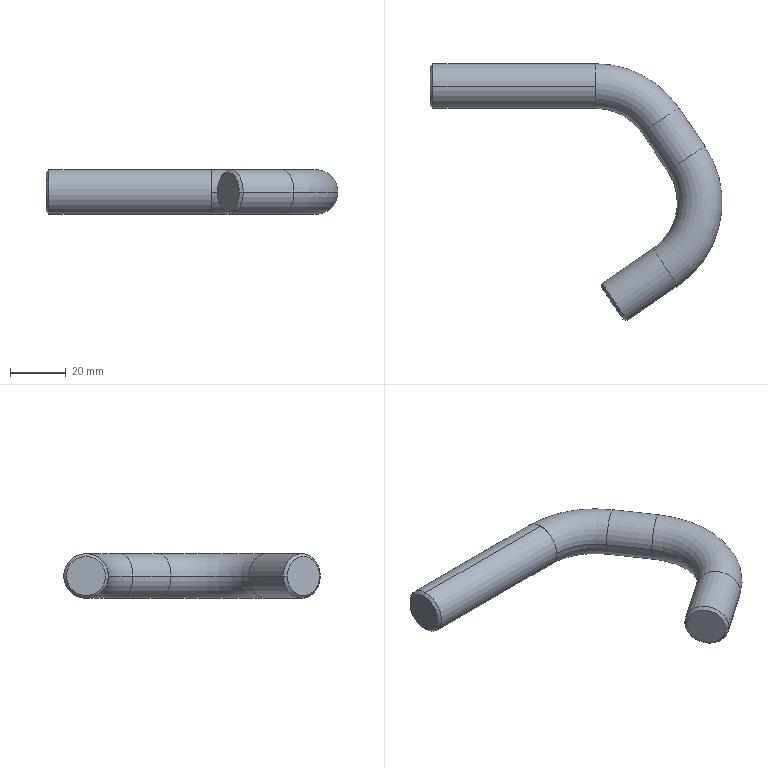Part | SolidWorks | features Chamfer 2, WeldMemberFeat 1, WeldmentFeature 1 | 5 solids | 24 faces | box 104.462 x 91.811 x 16 mm | volume 34123 mm3 | plane 10 | cylinder 6 | cone 4 | torus 4 | commonest cylinder face diameters 16 x6
STEP:
#1=CARTESIAN_POINT('',(0.,0.,7.));
#2=VERTEX_POINT('',#1);
#3=CARTESIAN_POINT('',(0.,0.,-7.));
#4=VERTEX_POINT('',#3);
#5=CARTESIAN_POINT('',(0.,0.,0.));
#6=DIRECTION('',(-1.,0.,0.));
#7=DIRECTION('',(0.,0.,1.));
#8=AXIS2_PLACEMENT_3D('',#5,#6,#7);
#9=CIRCLE('',#8,7.);
#10=EDGE_CURVE('',#2,#4,#9,.T.);
#11=ORIENTED_EDGE('',*,*,#10,.F.);
#12=CARTESIAN_POINT('',(1.,0.,8.));
#13=VERTEX_POINT('',#12);
#14=CARTESIAN_POINT('',(0.,0.,7.));
#15=DIRECTION('',(0.7071,0.,0.7071));
#16=VECTOR('',#15,1000.);
#17=LINE('',#14,#16);
#18=EDGE_CURVE('',#2,#13,#17,.T.);
#19=ORIENTED_EDGE('',*,*,#18,.T.);
#20=CARTESIAN_POINT('',(1.,0.,-8.));
#21=VERTEX_POINT('',#20);
#22=CARTESIAN_POINT('',(1.,0.,0.));
#23=DIRECTION('',(1.,0.,0.));
#24=DIRECTION('',(0.,0.,1.));
#25=AXIS2_PLACEMENT_3D('',#22,#23,#24);
#26=CIRCLE('',#25,8.);
#27=EDGE_CURVE('',#21,#13,#26,.T.);
#28=ORIENTED_EDGE('',*,*,#27,.F.);
#29=CARTESIAN_POINT('',(0.,0.,-7.));
#30=DIRECTION('',(0.7071,0.,-0.7071));
#31=VECTOR('',#30,1000.);
#32=LINE('',#29,#31);
#33=EDGE_CURVE('',#4,#21,#32,.T.);
#34=ORIENTED_EDGE('',*,*,#33,.F.);
#35=EDGE_LOOP('',(#11,#19,#28,#34));
#36=FACE_OUTER_BOUND('',#35,.T.);
#37=CARTESIAN_POINT('',(0.,0.,0.));
#38=DIRECTION('',(1.,0.,0.));
#39=DIRECTION('',(0.,0.,-1.));
#40=AXIS2_PLACEMENT_3D('',#37,#38,#39);
#41=CONICAL_SURFACE('',#40,7.,0.7854);
#42=ADVANCED_FACE('',(#36),#41,.T.);
#43=ORIENTED_EDGE('',*,*,#27,.T.);
#44=CARTESIAN_POINT('',(59.174,0.,8.));
#45=VERTEX_POINT('',#44);
#46=CARTESIAN_POINT('',(0.,0.,8.));
#47=DIRECTION('',(1.,0.,0.));
#48=VECTOR('',#47,1000.);
#49=LINE('',#46,#48);
#50=EDGE_CURVE('',#13,#45,#49,.T.);
#51=ORIENTED_EDGE('',*,*,#50,.T.);
#52=CARTESIAN_POINT('',(59.174,0.,-8.));
#53=VERTEX_POINT('',#52);
#54=CARTESIAN_POINT('',(59.174,0.,0.));
#55=DIRECTION('',(-1.,0.,0.));
#56=DIRECTION('',(0.,0.,1.));
#57=AXIS2_PLACEMENT_3D('',#54,#55,#56);
#58=CIRCLE('',#57,8.);
#59=EDGE_CURVE('',#45,#53,#58,.T.);
#60=ORIENTED_EDGE('',*,*,#59,.T.);
#61=CARTESIAN_POINT('',(0.,0.,-8.));
#62=DIRECTION('',(1.,0.,0.));
#63=VECTOR('',#62,1000.);
#64=LINE('',#61,#63);
#65=EDGE_CURVE('',#21,#53,#64,.T.);
#66=ORIENTED_EDGE('',*,*,#65,.F.);
#67=EDGE_LOOP('',(#43,#51,#60,#66));
#68=FACE_OUTER_BOUND('',#67,.T.);
#69=CARTESIAN_POINT('',(0.,0.,0.));
#70=DIRECTION('',(1.,0.,0.));
#71=DIRECTION('',(0.,0.,-1.));
#72=AXIS2_PLACEMENT_3D('',#69,#70,#71);
#73=CYLINDRICAL_SURFACE('',#72,8.);
#74=ADVANCED_FACE('',(#68),#73,.T.);
#75=ORIENTED_EDGE('',*,*,#50,.F.);
#76=CARTESIAN_POINT('',(1.,0.,0.));
#77=DIRECTION('',(1.,0.,0.));
#78=DIRECTION('',(0.,0.,1.));
#79=AXIS2_PLACEMENT_3D('',#76,#77,#78);
#80=CIRCLE('',#79,8.);
#81=EDGE_CURVE('',#13,#21,#80,.T.);
#82=ORIENTED_EDGE('',*,*,#81,.T.);
#83=ORIENTED_EDGE('',*,*,#65,.T.);
#84=CARTESIAN_POINT('',(59.174,0.,0.));
#85=DIRECTION('',(-1.,0.,0.));
#86=DIRECTION('',(0.,0.,1.));
#87=AXIS2_PLACEMENT_3D('',#84,#85,#86);
#88=CIRCLE('',#87,8.);
#89=EDGE_CURVE('',#53,#45,#88,.T.);
#90=ORIENTED_EDGE('',*,*,#89,.T.);
#91=EDGE_LOOP('',(#75,#82,#83,#90));
#92=FACE_OUTER_BOUND('',#91,.T.);
#93=CARTESIAN_POINT('',(0.,0.,0.));
#94=DIRECTION('',(1.,0.,0.));
#95=DIRECTION('',(0.,0.,-1.));
#96=AXIS2_PLACEMENT_3D('',#93,#94,#95);
#97=CYLINDRICAL_SURFACE('',#96,8.);
#98=ADVANCED_FACE('',(#92),#97,.T.);
#99=CARTESIAN_POINT('',(0.,0.,0.));
#100=DIRECTION('',(-1.,0.,0.));
#101=DIRECTION('',(0.,0.,1.));
#102=AXIS2_PLACEMENT_3D('',#99,#100,#101);
#103=CIRCLE('',#102,7.);
#104=EDGE_CURVE('',#4,#2,#103,.T.);
#105=ORIENTED_EDGE('',*,*,#104,.T.);
#106=ORIENTED_EDGE('',*,*,#10,.T.);
#107=EDGE_LOOP('',(#105,#106));
#108=FACE_OUTER_BOUND('',#107,.T.);
#109=CARTESIAN_POINT('',(0.,0.,0.));
#110=DIRECTION('',(-1.,0.,0.));
#111=DIRECTION('',(0.,0.,1.));
#112=AXIS2_PLACEMENT_3D('',#109,#110,#111);
#113=PLANE('',#112);
#114=ADVANCED_FACE('',(#108),#113,.T.);
#115=ORIENTED_EDGE('',*,*,#89,.F.);
#116=ORIENTED_EDGE('',*,*,#59,.F.);
#117=EDGE_LOOP('',(#115,#116));
#118=FACE_OUTER_BOUND('',#117,.T.);
#119=CARTESIAN_POINT('',(59.174,0.,0.));
#120=DIRECTION('',(-1.,0.,0.));
#121=DIRECTION('',(0.,0.,1.));
#122=AXIS2_PLACEMENT_3D('',#119,#120,#121);
#123=PLANE('',#122);
#124=ADVANCED_FACE('',(#118),#123,.F.);
#125=ORIENTED_EDGE('',*,*,#18,.F.);
#126=ORIENTED_EDGE('',*,*,#104,.F.);
#127=ORIENTED_EDGE('',*,*,#33,.T.);
#128=ORIENTED_EDGE('',*,*,#81,.F.);
#129=EDGE_LOOP('',(#125,#126,#127,#128));
#130=FACE_OUTER_BOUND('',#129,.T.);
#131=CARTESIAN_POINT('',(0.,0.,0.));
#132=DIRECTION('',(1.,0.,0.));
#133=DIRECTION('',(0.,0.,-1.));
#134=AXIS2_PLACEMENT_3D('',#131,#132,#133);
#135=CONICAL_SURFACE('',#134,7.,0.7854);
#136=ADVANCED_FACE('',(#130),#135,.T.);
#137=CLOSED_SHELL('',(#42,#74,#98,#114,#124,#136));
#138=MANIFOLD_SOLID_BREP('',#137);
#139=CARTESIAN_POINT('',(59.174,8.,0.));
#140=VERTEX_POINT('',#139);
#141=CARTESIAN_POINT('',(59.174,-8.,0.));
#142=VERTEX_POINT('',#141);
#143=CARTESIAN_POINT('',(59.174,0.,0.));
#144=DIRECTION('',(-1.,0.,0.));
#145=DIRECTION('',(0.,0.,1.));
#146=AXIS2_PLACEMENT_3D('',#143,#144,#145);
#147=CIRCLE('',#146,8.);
#148=EDGE_CURVE('',#140,#142,#147,.T.);
#149=ORIENTED_EDGE('',*,*,#148,.F.);
#150=CARTESIAN_POINT('',(88.95,-7.767,0.));
#151=VERTEX_POINT('',#150);
#152=CARTESIAN_POINT('',(59.174,-28.,0.));
#153=DIRECTION('',(0.,0.,-1.));
#154=DIRECTION('',(-1.,0.,0.));
#155=AXIS2_PLACEMENT_3D('',#152,#153,#154);
#156=CIRCLE('',#155,36.);
#157=EDGE_CURVE('',#140,#151,#156,.T.);
#158=ORIENTED_EDGE('',*,*,#157,.T.);
#159=CARTESIAN_POINT('',(75.716,-16.759,0.));
#160=VERTEX_POINT('',#159);
#161=CARTESIAN_POINT('',(82.333,-12.263,0.));
#162=DIRECTION('',(-0.562,0.8271,0.));
#163=DIRECTION('',(0.,0.,1.));
#164=AXIS2_PLACEMENT_3D('',#161,#162,#163);
#165=CIRCLE('',#164,8.);
#166=EDGE_CURVE('',#151,#160,#165,.T.);
#167=ORIENTED_EDGE('',*,*,#166,.T.);
#168=CARTESIAN_POINT('',(59.174,-28.,0.));
#169=DIRECTION('',(0.,0.,-1.));
#170=DIRECTION('',(-1.,0.,0.));
#171=AXIS2_PLACEMENT_3D('',#168,#169,#170);
#172=CIRCLE('',#171,20.);
#173=EDGE_CURVE('',#142,#160,#172,.T.);
#174=ORIENTED_EDGE('',*,*,#173,.F.);
#175=EDGE_LOOP('',(#149,#158,#167,#174));
#176=FACE_OUTER_BOUND('',#175,.T.);
#177=CARTESIAN_POINT('',(59.174,-28.,0.));
#178=DIRECTION('',(0.,0.,-1.));
#179=DIRECTION('',(-1.,0.,0.));
#180=AXIS2_PLACEMENT_3D('',#177,#178,#179);
#181=TOROIDAL_SURFACE('',#180,28.,8.);
#182=ADVANCED_FACE('',(#176),#181,.T.);
#183=CARTESIAN_POINT('',(59.174,0.,0.));
#184=DIRECTION('',(-1.,0.,0.));
#185=DIRECTION('',(0.,0.,1.));
#186=AXIS2_PLACEMENT_3D('',#183,#184,#185);
#187=CIRCLE('',#186,8.);
#188=EDGE_CURVE('',#142,#140,#187,.T.);
#189=ORIENTED_EDGE('',*,*,#188,.T.);
#190=ORIENTED_EDGE('',*,*,#148,.T.);
#191=EDGE_LOOP('',(#189,#190));
#192=FACE_OUTER_BOUND('',#191,.T.);
#193=CARTESIAN_POINT('',(59.174,0.,0.));
#194=DIRECTION('',(-1.,0.,0.));
#195=DIRECTION('',(0.,0.,1.));
#196=AXIS2_PLACEMENT_3D('',#193,#194,#195);
#197=PLANE('',#196);
#198=ADVANCED_FACE('',(#192),#197,.T.);
#199=ORIENTED_EDGE('',*,*,#157,.F.);
#200=ORIENTED_EDGE('',*,*,#188,.F.);
#201=ORIENTED_EDGE('',*,*,#173,.T.);
#202=CARTESIAN_POINT('',(82.333,-12.263,0.));
#203=DIRECTION('',(-0.562,0.8271,0.));
#204=DIRECTION('',(0.,0.,1.));
#205=AXIS2_PLACEMENT_3D('',#202,#203,#204);
#206=CIRCLE('',#205,8.);
#207=EDGE_CURVE('',#160,#151,#206,.T.);
#208=ORIENTED_EDGE('',*,*,#207,.T.);
#209=EDGE_LOOP('',(#199,#200,#201,#208));
#210=FACE_OUTER_BOUND('',#209,.T.);
#211=CARTESIAN_POINT('',(59.174,-28.,0.));
#212=DIRECTION('',(0.,0.,-1.));
#213=DIRECTION('',(-1.,0.,0.));
#214=AXIS2_PLACEMENT_3D('',#211,#212,#213);
#215=TOROIDAL_SURFACE('',#214,28.,8.);
#216=ADVANCED_FACE('',(#210),#215,.T.);
#217=ORIENTED_EDGE('',*,*,#207,.F.);
#218=ORIENTED_EDGE('',*,*,#166,.F.);
#219=EDGE_LOOP('',(#217,#218));
#220=FACE_OUTER_BOUND('',#219,.T.);
#221=CARTESIAN_POINT('',(82.333,-12.263,0.));
#222=DIRECTION('',(-0.562,0.8271,0.));
#223=DIRECTION('',(0.,0.,1.));
#224=AXIS2_PLACEMENT_3D('',#221,#222,#223);
#225=PLANE('',#224);
#226=ADVANCED_FACE('',(#220),#225,.F.);
#227=CLOSED_SHELL('',(#182,#198,#216,#226));
#228=MANIFOLD_SOLID_BREP('',#227);
#229=CARTESIAN_POINT('',(75.716,-16.759,0.));
#230=VERTEX_POINT('',#229);
#231=CARTESIAN_POINT('',(88.95,-7.767,0.));
#232=VERTEX_POINT('',#231);
#233=CARTESIAN_POINT('',(82.333,-12.263,0.));
#234=DIRECTION('',(-0.562,0.8271,0.));
#235=DIRECTION('',(0.,0.,1.));
#236=AXIS2_PLACEMENT_3D('',#233,#234,#235);
#237=CIRCLE('',#236,8.);
#238=EDGE_CURVE('',#230,#232,#237,.T.);
#239=ORIENTED_EDGE('',*,*,#238,.F.);
#240=CARTESIAN_POINT('',(85.005,-30.429,0.));
#241=VERTEX_POINT('',#240);
#242=CARTESIAN_POINT('',(75.716,-16.759,0.));
#243=DIRECTION('',(0.562,-0.8271,0.));
#244=VECTOR('',#243,1000.);
#245=LINE('',#242,#244);
#246=EDGE_CURVE('',#230,#241,#245,.T.);
#247=ORIENTED_EDGE('',*,*,#246,.T.);
#248=CARTESIAN_POINT('',(98.239,-21.437,0.));
#249=VERTEX_POINT('',#248);
#250=CARTESIAN_POINT('',(91.622,-25.933,0.));
#251=DIRECTION('',(-0.562,0.8271,0.));
#252=DIRECTION('',(0.,0.,1.));
#253=AXIS2_PLACEMENT_3D('',#250,#251,#252);
#254=CIRCLE('',#253,8.);
#255=EDGE_CURVE('',#241,#249,#254,.T.);
#256=ORIENTED_EDGE('',*,*,#255,.T.);
#257=CARTESIAN_POINT('',(88.95,-7.767,0.));
#258=DIRECTION('',(0.562,-0.8271,0.));
#259=VECTOR('',#258,1000.);
#260=LINE('',#257,#259);
#261=EDGE_CURVE('',#232,#249,#260,.T.);
#262=ORIENTED_EDGE('',*,*,#261,.F.);
#263=EDGE_LOOP('',(#239,#247,#256,#262));
#264=FACE_OUTER_BOUND('',#263,.T.);
#265=CARTESIAN_POINT('',(82.333,-12.263,0.));
#266=DIRECTION('',(0.562,-0.8271,0.));
#267=DIRECTION('',(0.8271,0.562,0.));
#268=AXIS2_PLACEMENT_3D('',#265,#266,#267);
#269=CYLINDRICAL_SURFACE('',#268,8.);
#270=ADVANCED_FACE('',(#264),#269,.T.);
#271=ORIENTED_EDGE('',*,*,#246,.F.);
#272=CARTESIAN_POINT('',(82.333,-12.263,0.));
#273=DIRECTION('',(-0.562,0.8271,0.));
#274=DIRECTION('',(0.,0.,1.));
#275=AXIS2_PLACEMENT_3D('',#272,#273,#274);
#276=CIRCLE('',#275,8.);
#277=EDGE_CURVE('',#232,#230,#276,.T.);
#278=ORIENTED_EDGE('',*,*,#277,.F.);
#279=ORIENTED_EDGE('',*,*,#261,.T.);
#280=CARTESIAN_POINT('',(91.622,-25.933,0.));
#281=DIRECTION('',(-0.562,0.8271,0.));
#282=DIRECTION('',(0.,0.,1.));
#283=AXIS2_PLACEMENT_3D('',#280,#281,#282);
#284=CIRCLE('',#283,8.);
#285=EDGE_CURVE('',#249,#241,#284,.T.);
#286=ORIENTED_EDGE('',*,*,#285,.T.);
#287=EDGE_LOOP('',(#271,#278,#279,#286));
#288=FACE_OUTER_BOUND('',#287,.T.);
#289=CARTESIAN_POINT('',(82.333,-12.263,0.));
#290=DIRECTION('',(0.562,-0.8271,0.));
#291=DIRECTION('',(0.8271,0.562,0.));
#292=AXIS2_PLACEMENT_3D('',#289,#290,#291);
#293=CYLINDRICAL_SURFACE('',#292,8.);
#294=ADVANCED_FACE('',(#288),#293,.T.);
#295=ORIENTED_EDGE('',*,*,#277,.T.);
#296=ORIENTED_EDGE('',*,*,#238,.T.);
#297=EDGE_LOOP('',(#295,#296));
#298=FACE_OUTER_BOUND('',#297,.T.);
#299=CARTESIAN_POINT('',(82.333,-12.263,0.));
#300=DIRECTION('',(-0.562,0.8271,0.));
#301=DIRECTION('',(0.,0.,1.));
#302=AXIS2_PLACEMENT_3D('',#299,#300,#301);
#303=PLANE('',#302);
#304=ADVANCED_FACE('',(#298),#303,.T.);
#305=ORIENTED_EDGE('',*,*,#285,.F.);
#306=ORIENTED_EDGE('',*,*,#255,.F.);
#307=EDGE_LOOP('',(#305,#306));
#308=FACE_OUTER_BOUND('',#307,.T.);
#309=CARTESIAN_POINT('',(91.622,-25.933,0.));
#310=DIRECTION('',(-0.562,0.8271,0.));
#311=DIRECTION('',(0.,0.,1.));
#312=AXIS2_PLACEMENT_3D('',#309,#310,#311);
#313=PLANE('',#312);
#314=ADVANCED_FACE('',(#308),#313,.F.);
#315=CLOSED_SHELL('',(#270,#294,#304,#314));
#316=MANIFOLD_SOLID_BREP('',#315);
#317=CARTESIAN_POINT('',(98.239,-21.437,0.));
#318=VERTEX_POINT('',#317);
#319=CARTESIAN_POINT('',(85.005,-30.429,0.));
#320=VERTEX_POINT('',#319);
#321=CARTESIAN_POINT('',(91.622,-25.933,0.));
#322=DIRECTION('',(-0.562,0.8271,0.));
#323=DIRECTION('',(0.,0.,1.));
#324=AXIS2_PLACEMENT_3D('',#321,#322,#323);
#325=CIRCLE('',#324,8.);
#326=EDGE_CURVE('',#318,#320,#325,.T.);
#327=ORIENTED_EDGE('',*,*,#326,.F.);
#328=CARTESIAN_POINT('',(88.695,-71.446,0.));
#329=VERTEX_POINT('',#328);
#330=CARTESIAN_POINT('',(68.462,-41.67,0.));
#331=DIRECTION('',(0.,0.,-1.));
#332=DIRECTION('',(-1.,0.,0.));
#333=AXIS2_PLACEMENT_3D('',#330,#331,#332);
#334=CIRCLE('',#333,36.);
#335=EDGE_CURVE('',#318,#329,#334,.T.);
#336=ORIENTED_EDGE('',*,*,#335,.T.);
#337=CARTESIAN_POINT('',(79.703,-58.212,0.));
#338=VERTEX_POINT('',#337);
#339=CARTESIAN_POINT('',(84.199,-64.829,0.));
#340=DIRECTION('',(0.8271,0.562,0.));
#341=DIRECTION('',(0.,0.,1.));
#342=AXIS2_PLACEMENT_3D('',#339,#340,#341);
#343=CIRCLE('',#342,8.);
#344=EDGE_CURVE('',#329,#338,#343,.T.);
#345=ORIENTED_EDGE('',*,*,#344,.T.);
#346=CARTESIAN_POINT('',(68.462,-41.67,0.));
#347=DIRECTION('',(0.,0.,-1.));
#348=DIRECTION('',(-1.,0.,0.));
#349=AXIS2_PLACEMENT_3D('',#346,#347,#348);
#350=CIRCLE('',#349,20.);
#351=EDGE_CURVE('',#320,#338,#350,.T.);
#352=ORIENTED_EDGE('',*,*,#351,.F.);
#353=EDGE_LOOP('',(#327,#336,#345,#352));
#354=FACE_OUTER_BOUND('',#353,.T.);
#355=CARTESIAN_POINT('',(68.462,-41.67,0.));
#356=DIRECTION('',(0.,0.,-1.));
#357=DIRECTION('',(-1.,0.,0.));
#358=AXIS2_PLACEMENT_3D('',#355,#356,#357);
#359=TOROIDAL_SURFACE('',#358,28.,8.);
#360=ADVANCED_FACE('',(#354),#359,.T.);
#361=CARTESIAN_POINT('',(91.622,-25.933,0.));
#362=DIRECTION('',(-0.562,0.8271,0.));
#363=DIRECTION('',(0.,0.,1.));
#364=AXIS2_PLACEMENT_3D('',#361,#362,#363);
#365=CIRCLE('',#364,8.);
#366=EDGE_CURVE('',#320,#318,#365,.T.);
#367=ORIENTED_EDGE('',*,*,#366,.T.);
#368=ORIENTED_EDGE('',*,*,#326,.T.);
#369=EDGE_LOOP('',(#367,#368));
#370=FACE_OUTER_BOUND('',#369,.T.);
#371=CARTESIAN_POINT('',(91.622,-25.933,0.));
#372=DIRECTION('',(-0.562,0.8271,0.));
#373=DIRECTION('',(0.,0.,1.));
#374=AXIS2_PLACEMENT_3D('',#371,#372,#373);
#375=PLANE('',#374);
#376=ADVANCED_FACE('',(#370),#375,.T.);
#377=ORIENTED_EDGE('',*,*,#335,.F.);
#378=ORIENTED_EDGE('',*,*,#366,.F.);
#379=ORIENTED_EDGE('',*,*,#351,.T.);
#380=CARTESIAN_POINT('',(84.199,-64.829,0.));
#381=DIRECTION('',(0.8271,0.562,0.));
#382=DIRECTION('',(0.,0.,1.));
#383=AXIS2_PLACEMENT_3D('',#380,#381,#382);
#384=CIRCLE('',#383,8.);
#385=EDGE_CURVE('',#338,#329,#384,.T.);
#386=ORIENTED_EDGE('',*,*,#385,.T.);
#387=EDGE_LOOP('',(#377,#378,#379,#386));
#388=FACE_OUTER_BOUND('',#387,.T.);
#389=CARTESIAN_POINT('',(68.462,-41.67,0.));
#390=DIRECTION('',(0.,0.,-1.));
#391=DIRECTION('',(-1.,0.,0.));
#392=AXIS2_PLACEMENT_3D('',#389,#390,#391);
#393=TOROIDAL_SURFACE('',#392,28.,8.);
#394=ADVANCED_FACE('',(#388),#393,.T.);
#395=ORIENTED_EDGE('',*,*,#385,.F.);
#396=ORIENTED_EDGE('',*,*,#344,.F.);
#397=EDGE_LOOP('',(#395,#396));
#398=FACE_OUTER_BOUND('',#397,.T.);
#399=CARTESIAN_POINT('',(84.199,-64.829,0.));
#400=DIRECTION('',(0.8271,0.562,0.));
#401=DIRECTION('',(0.,0.,1.));
#402=AXIS2_PLACEMENT_3D('',#399,#400,#401);
#403=PLANE('',#402);
#404=ADVANCED_FACE('',(#398),#403,.F.);
#405=CLOSED_SHELL('',(#360,#376,#394,#404));
#406=MANIFOLD_SOLID_BREP('',#405);
#407=CARTESIAN_POINT('',(69.109,-83.546,0.));
#408=VERTEX_POINT('',#407);
#409=CARTESIAN_POINT('',(61.241,-71.966,0.));
#410=VERTEX_POINT('',#409);
#411=CARTESIAN_POINT('',(65.175,-77.756,0.));
#412=DIRECTION('',(-0.8271,-0.562,0.));
#413=DIRECTION('',(-0.562,0.8271,0.));
#414=AXIS2_PLACEMENT_3D('',#411,#412,#413);
#415=CIRCLE('',#414,7.);
#416=EDGE_CURVE('',#408,#410,#415,.T.);
#417=ORIENTED_EDGE('',*,*,#416,.F.);
#418=CARTESIAN_POINT('',(70.499,-83.811,0.));
#419=VERTEX_POINT('',#418);
#420=CARTESIAN_POINT('',(70.499,-83.811,0.));
#421=DIRECTION('',(0.9823,-0.1874,0.));
#422=VECTOR('',#421,1000.);
#423=LINE('',#420,#422);
#424=EDGE_CURVE('',#408,#419,#423,.T.);
#425=ORIENTED_EDGE('',*,*,#424,.T.);
#426=CARTESIAN_POINT('',(61.506,-70.577,0.));
#427=VERTEX_POINT('',#426);
#428=CARTESIAN_POINT('',(66.002,-77.194,0.));
#429=DIRECTION('',(0.8271,0.562,0.));
#430=DIRECTION('',(-0.562,0.8271,0.));
#431=AXIS2_PLACEMENT_3D('',#428,#429,#430);
#432=CIRCLE('',#431,8.);
#433=EDGE_CURVE('',#427,#419,#432,.T.);
#434=ORIENTED_EDGE('',*,*,#433,.F.);
#435=CARTESIAN_POINT('',(61.506,-70.577,0.));
#436=DIRECTION('',(0.1874,0.9823,0.));
#437=VECTOR('',#436,1000.);
#438=LINE('',#435,#437);
#439=EDGE_CURVE('',#410,#427,#438,.T.);
#440=ORIENTED_EDGE('',*,*,#439,.F.);
#441=EDGE_LOOP('',(#417,#425,#434,#440));
#442=FACE_OUTER_BOUND('',#441,.T.);
#443=CARTESIAN_POINT('',(66.002,-77.194,0.));
#444=DIRECTION('',(0.8271,0.562,0.));
#445=DIRECTION('',(-0.562,0.8271,0.));
#446=AXIS2_PLACEMENT_3D('',#443,#444,#445);
#447=CONICAL_SURFACE('',#446,8.,0.7854);
#448=ADVANCED_FACE('',(#442),#447,.T.);
#449=CARTESIAN_POINT('',(79.703,-58.212,0.));
#450=VERTEX_POINT('',#449);
#451=CARTESIAN_POINT('',(88.695,-71.446,0.));
#452=VERTEX_POINT('',#451);
#453=CARTESIAN_POINT('',(84.199,-64.829,0.));
#454=DIRECTION('',(0.8271,0.562,0.));
#455=DIRECTION('',(0.,0.,1.));
#456=AXIS2_PLACEMENT_3D('',#453,#454,#455);
#457=CIRCLE('',#456,8.);
#458=EDGE_CURVE('',#450,#452,#457,.T.);
#459=ORIENTED_EDGE('',*,*,#458,.F.);
#460=CARTESIAN_POINT('',(79.703,-58.212,0.));
#461=DIRECTION('',(-0.8271,-0.562,0.));
#462=VECTOR('',#461,1000.);
#463=LINE('',#460,#462);
#464=EDGE_CURVE('',#450,#427,#463,.T.);
#465=ORIENTED_EDGE('',*,*,#464,.T.);
#466=ORIENTED_EDGE('',*,*,#433,.T.);
#467=CARTESIAN_POINT('',(88.695,-71.446,0.));
#468=DIRECTION('',(-0.8271,-0.562,0.));
#469=VECTOR('',#468,1000.);
#470=LINE('',#467,#469);
#471=EDGE_CURVE('',#452,#419,#470,.T.);
#472=ORIENTED_EDGE('',*,*,#471,.F.);
#473=EDGE_LOOP('',(#459,#465,#466,#472));
#474=FACE_OUTER_BOUND('',#473,.T.);
#475=CARTESIAN_POINT('',(84.199,-64.829,0.));
#476=DIRECTION('',(-0.8271,-0.562,0.));
#477=DIRECTION('',(0.562,-0.8271,0.));
#478=AXIS2_PLACEMENT_3D('',#475,#476,#477);
#479=CYLINDRICAL_SURFACE('',#478,8.);
#480=ADVANCED_FACE('',(#474),#479,.T.);
#481=ORIENTED_EDGE('',*,*,#464,.F.);
#482=CARTESIAN_POINT('',(84.199,-64.829,0.));
#483=DIRECTION('',(0.8271,0.562,0.));
#484=DIRECTION('',(0.,0.,1.));
#485=AXIS2_PLACEMENT_3D('',#482,#483,#484);
#486=CIRCLE('',#485,8.);
#487=EDGE_CURVE('',#452,#450,#486,.T.);
#488=ORIENTED_EDGE('',*,*,#487,.F.);
#489=ORIENTED_EDGE('',*,*,#471,.T.);
#490=CARTESIAN_POINT('',(66.002,-77.194,0.));
#491=DIRECTION('',(0.8271,0.562,0.));
#492=DIRECTION('',(-0.562,0.8271,0.));
#493=AXIS2_PLACEMENT_3D('',#490,#491,#492);
#494=CIRCLE('',#493,8.);
#495=EDGE_CURVE('',#419,#427,#494,.T.);
#496=ORIENTED_EDGE('',*,*,#495,.T.);
#497=EDGE_LOOP('',(#481,#488,#489,#496));
#498=FACE_OUTER_BOUND('',#497,.T.);
#499=CARTESIAN_POINT('',(84.199,-64.829,0.));
#500=DIRECTION('',(-0.8271,-0.562,0.));
#501=DIRECTION('',(0.562,-0.8271,0.));
#502=AXIS2_PLACEMENT_3D('',#499,#500,#501);
#503=CYLINDRICAL_SURFACE('',#502,8.);
#504=ADVANCED_FACE('',(#498),#503,.T.);
#505=ORIENTED_EDGE('',*,*,#487,.T.);
#506=ORIENTED_EDGE('',*,*,#458,.T.);
#507=EDGE_LOOP('',(#505,#506));
#508=FACE_OUTER_BOUND('',#507,.T.);
#509=CARTESIAN_POINT('',(84.199,-64.829,0.));
#510=DIRECTION('',(0.8271,0.562,0.));
#511=DIRECTION('',(0.,0.,1.));
#512=AXIS2_PLACEMENT_3D('',#509,#510,#511);
#513=PLANE('',#512);
#514=ADVANCED_FACE('',(#508),#513,.T.);
#515=CARTESIAN_POINT('',(65.175,-77.756,0.));
#516=DIRECTION('',(-0.8271,-0.562,0.));
#517=DIRECTION('',(-0.562,0.8271,0.));
#518=AXIS2_PLACEMENT_3D('',#515,#516,#517);
#519=CIRCLE('',#518,7.);
#520=EDGE_CURVE('',#410,#408,#519,.T.);
#521=ORIENTED_EDGE('',*,*,#520,.T.);
#522=ORIENTED_EDGE('',*,*,#416,.T.);
#523=EDGE_LOOP('',(#521,#522));
#524=FACE_OUTER_BOUND('',#523,.T.);
#525=CARTESIAN_POINT('',(65.175,-77.756,0.));
#526=DIRECTION('',(0.8271,0.562,0.));
#527=DIRECTION('',(0.,0.,1.));
#528=AXIS2_PLACEMENT_3D('',#525,#526,#527);
#529=PLANE('',#528);
#530=ADVANCED_FACE('',(#524),#529,.F.);
#531=ORIENTED_EDGE('',*,*,#424,.F.);
#532=ORIENTED_EDGE('',*,*,#520,.F.);
#533=ORIENTED_EDGE('',*,*,#439,.T.);
#534=ORIENTED_EDGE('',*,*,#495,.F.);
#535=EDGE_LOOP('',(#531,#532,#533,#534));
#536=FACE_OUTER_BOUND('',#535,.T.);
#537=CARTESIAN_POINT('',(66.002,-77.194,0.));
#538=DIRECTION('',(0.8271,0.562,0.));
#539=DIRECTION('',(-0.562,0.8271,0.));
#540=AXIS2_PLACEMENT_3D('',#537,#538,#539);
#541=CONICAL_SURFACE('',#540,8.,0.7854);
#542=ADVANCED_FACE('',(#536),#541,.T.);
#543=CLOSED_SHELL('',(#448,#480,#504,#514,#530,#542));
#544=MANIFOLD_SOLID_BREP('',#543);
#545=CARTESIAN_POINT('',(0.,0.,0.));
#546=DIRECTION('',(0.,0.,1.));
#547=DIRECTION('',(1.,0.,0.));
#548=AXIS2_PLACEMENT_3D('',#545,#546,#547);
#549=(LENGTH_UNIT()NAMED_UNIT(*)SI_UNIT(.MILLI.,.METRE.));
#550=UNCERTAINTY_MEASURE_WITH_UNIT(LENGTH_MEASURE(0.00001),#549,'','');
#551=(NAMED_UNIT(*)PLANE_ANGLE_UNIT()SI_UNIT($,.RADIAN.));
#552=(NAMED_UNIT(*)SI_UNIT($,.STERADIAN.)SOLID_ANGLE_UNIT());
#553=(GEOMETRIC_REPRESENTATION_CONTEXT(3)GLOBAL_UNCERTAINTY_ASSIGNED_CONTEXT((#550))GLOBAL_UNIT_ASSIGNED_CONTEXT((#549,#551,#552))REPRESENTATION_CONTEXT('',''));
#554=ADVANCED_BREP_SHAPE_REPRESENTATION('',(#138,#228,#316,#406,#544,#548),#553);